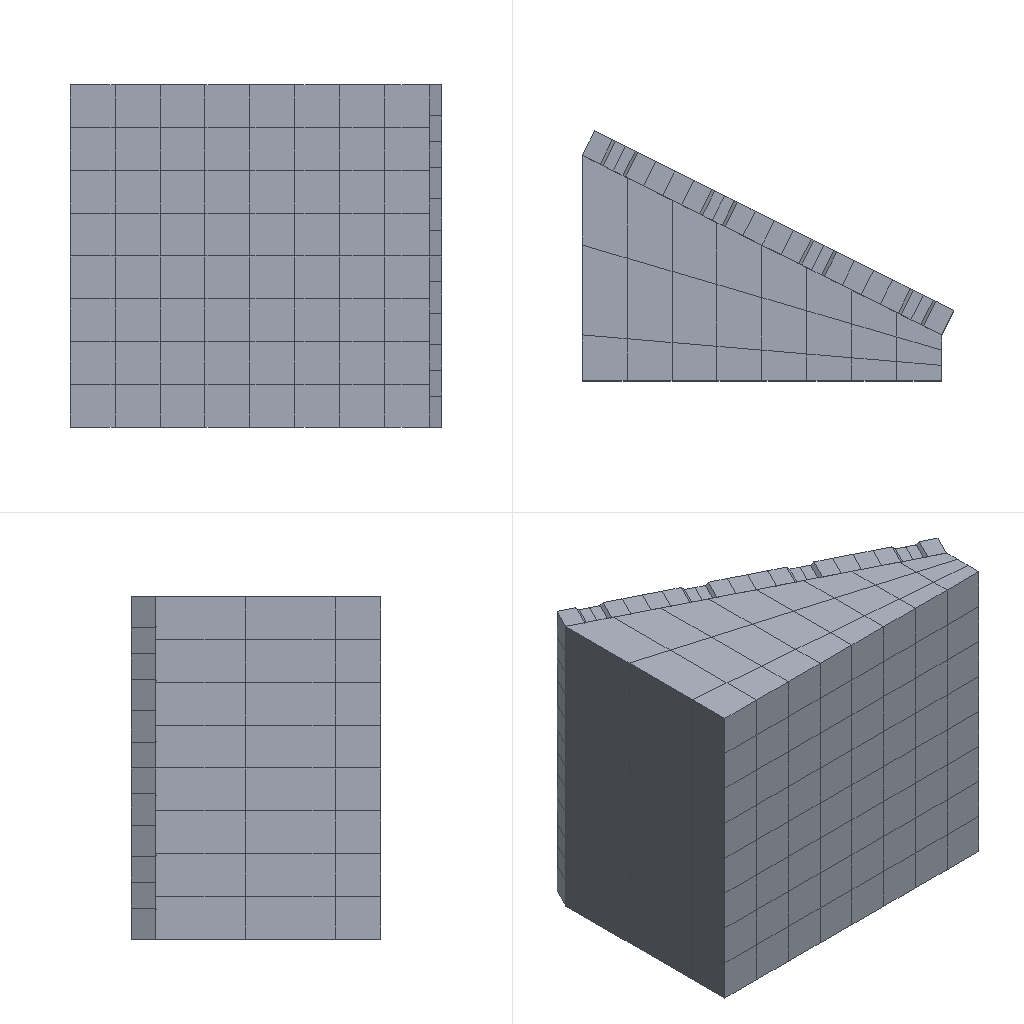Simulation study | abaqus
Set-up summary:
category,name,step,type,value,unit,region
solver,abaqus
solver,version,,,Abaqus/Standard 2020
units,not stated in the deck,,not stated
analysis,deck,,transient,transient
load_step,Step-2,Step-2,transient
load_step,requested,,,1
mesh,nodes,,,3205
mesh,elements,,,1224
element_type,C3D8R,,solid,1224
load,load commands in deck,,count,7
bc,support commands in deck,,count,7
material,HUNNINGTU,,in results
material,S,,in results
check,setup vs results,,match,"per instance, exact: element labels, types and connectivity; labels of the nodes the elements use; coordinates of those nodes at SINGLE_PRECISION in 15 of 31 instance(s)"
Abaqus input file, long lists of numbers shortened, first 402 of 1311 lines:
*Heading
** Job name: Job-2 Model name: Job-9-Copy
** Generated by: Abaqus/CAE 2020
*Preprint, echo=NO, model=NO, history=NO, contact=NO
**
** PARTS
**
*Part, name=BIKONGQIKUAI1
*Node
      1,  -23.409,         -15.,          12.
      2,  -23.409,  -10.17,          12.
** (128 more lines like these left out)
*Element, type=C3D8R
 1,  26,  33,  60,  27,  91,  98, 125,  92
 2,   1,   2,  44,  35,  66,  67, 109, 100
** (46 more lines like these left out)
*Nset, nset=SET-1, generate
   1,  130,    1
*Elset, elset=SET-1, generate
  1,  48,   1
** Section: Section-2-SET-1
*Solid Section, elset=SET-1, material=HUNNINGTU
,
*End Part
**
*Part, name=BIKONGQIKUAI1-COPY
*Node
      1,  0.1705,  -24.319,           0.
      2,  0.1705,  -5.681,           0.
** (62 more lines like these left out)
*Element, type=C3D8R
 1, 21,  3, 29, 25, 53, 35, 61, 57
 2, 22, 32, 30, 20, 54, 64, 62, 52
** (20 more lines like these left out)
*Nset, nset=SET-1, generate
  1,  64,   1
*Elset, elset=SET-1, generate
  1,  22,   1
** Section: Section-3-SET-1
*Solid Section, elset=SET-1, material=HUNNINGTU
,
*End Part
**
*Part, name=BIKONGQIKUAI1-COPY2
*Node
      1,   13.807,  -3.411,          12.
      2,   13.807,  -5.681,          12.
** (24 more lines like these left out)
*Element, type=C3D8R
1,  5, 18,  2,  1,  8, 24, 12, 13
2, 20,  3, 18,  5, 21, 23, 24,  8
** (4 more lines like these left out)
*Nset, nset=TIANCHONG, generate
  1,  26,   1
*Elset, elset=TIANCHONG, generate
 1,  6,  1
** Section: Section-4-TIANCHONG
*Solid Section, elset=TIANCHONG, material=HUNNINGTU
,
*End Part
**
*Part, name=PART-6
*Node
      1,  -157.419,   78.696,         150.
      2,  -137.741,   68.859,         150.
** (323 more lines like these left out)
*Element, type=C3D8R
  1,  82,  83,  92,  91,   1,   2,  11,  10
  2,  83,  84,  93,  92,   2,   3,  12,  11
** (190 more lines like these left out)
*Nset, nset=PART-6-REFPT_, internal
 325,
*Nset, nset=SET-2, generate
   1,  324,    1
*Elset, elset=SET-2, generate
   1,  192,    1
** Section: Section-1-SET-2
*Solid Section, elset=SET-2, material=S
,
*End Part
**
**
** ASSEMBLY
**
*Assembly, name=Assembly
**
*Instance, name=PART-6-1, part=PART-6
*End Instance
**
*Instance, name=BIKONGQIKUAI1-1, part=BIKONGQIKUAI1
-26.827, 13.414, 125.171
-26.827, 13.414, 125.171, -27.292, 14.167, 125.636, 106.047
*End Instance
**
*Instance, name=BIKONGQIKUAI1-COPY-1, part=BIKONGQIKUAI1-COPY
-48.579, 24.288, 150.171
-48.579, 24.288, 150.171, -49.045, 25.041, 150.636, 106.047
*End Instance
**
*Instance, name=BIKONGQIKUAI1-COPY2-1, part=BIKONGQIKUAI1-COPY2
-5.359, -10.734, 124.83
-5.359, -10.734, 124.83, -4.711, -10.333, 125.477, 223.65
*End Instance
**
*Instance, name=BIKONGQIKUAI1-1-LIN-1-2, part=BIKONGQIKUAI1
-26.827, 13.414, 75.171
-26.827, 13.414, 75.171, -27.292, 14.167, 75.636, 106.047
*End Instance
**
*Instance, name=BIKONGQIKUAI1-1-LIN-1-3, part=BIKONGQIKUAI1
-26.827, 13.414, 25.171
-26.827, 13.414, 25.171, -27.292, 14.167, 25.636, 106.047
*End Instance
**
*Instance, name=BIKONGQIKUAI1-1-LIN-2-1, part=BIKONGQIKUAI1
-48.579, 24.288, 100.17
-48.579, 24.288, 100.17, -49.045, 25.041, 100.635, 106.047
*End Instance
**
*Instance, name=BIKONGQIKUAI1-1-LIN-2-2, part=BIKONGQIKUAI1
-48.579, 24.288, 50.171
-48.579, 24.288, 50.171, -49.045, 25.041, 50.636, 106.047
*End Instance
**
*Instance, name=BIKONGQIKUAI1-1-LIN-2-3, part=BIKONGQIKUAI1
-70.331, 35.161, 25.17
-70.331, 35.161, 25.17, -70.797, 35.914, 25.635, 106.047
*End Instance
**
*Instance, name=BIKONGQIKUAI1-1-LIN-3-1, part=BIKONGQIKUAI1
-113.835, 56.909, 125.172
-113.835, 56.909, 125.172, -114.301, 57.662, 125.637, 106.047
*End Instance
**
*Instance, name=BIKONGQIKUAI1-1-LIN-3-2, part=BIKONGQIKUAI1
-92.083, 46.035, 100.171
-92.083, 46.035, 100.171, -92.549, 46.788, 100.636, 106.047
*End Instance
**
*Instance, name=BIKONGQIKUAI1-1-LIN-3-3, part=BIKONGQIKUAI1
-92.083, 46.035, 50.171
-92.083, 46.035, 50.171, -92.549, 46.788, 50.636, 106.047
*End Instance
**
*Instance, name=BIKONGQIKUAI1-1-LIN-4-1, part=BIKONGQIKUAI1
-113.835, 56.909, 75.17
-113.835, 56.909, 75.17, -114.301, 57.662, 75.635, 106.047
*End Instance
**
*Instance, name=BIKONGQIKUAI1-1-LIN-4-2, part=BIKONGQIKUAI1
-135.587, 67.782, 100.171
-135.587, 67.782, 100.171, -136.053, 68.535, 100.636, 106.047
*End Instance
**
*Instance, name=BIKONGQIKUAI1-1-LIN-4-3, part=BIKONGQIKUAI1
-157.34, 78.656, 125.172
-157.34, 78.656, 125.172, -157.805, 79.409, 125.637, 106.047
*End Instance
**
*Instance, name=BIKONGQIKUAI1-1-LIN-2-3-LIN-2-1, part=BIKONGQIKUAI1
-70.331, 35.161, 75.17
-70.331, 35.161, 75.17, -70.797, 35.914, 75.635, 106.047
*End Instance
**
*Instance, name=BIKONGQIKUAI1-1-LIN-2-3-LIN-3-1, part=BIKONGQIKUAI1
-70.331, 35.161, 125.17
-70.331, 35.161, 125.17, -70.797, 35.914, 125.635, 106.047
*End Instance
**
*Instance, name=BIKONGQIKUAI1-1-LIN-4-3-LIN-2-1, part=BIKONGQIKUAI1
-157.34, 78.656, 75.172
-157.34, 78.656, 75.172, -157.805, 79.409, 75.637, 106.047
*End Instance
**
*Instance, name=BIKONGQIKUAI1-1-LIN-4-3-LIN-3-1, part=BIKONGQIKUAI1
-157.34, 78.656, 25.172
-157.34, 78.656, 25.172, -157.805, 79.409, 25.637, 106.047
*End Instance
**
*Instance, name=BIKONGQIKUAI1-1-LIN-4-2-LIN-2-1, part=BIKONGQIKUAI1
-135.587, 67.782, 50.171
-135.587, 67.782, 50.171, -136.053, 68.535, 50.636, 106.047
*End Instance
**
*Instance, name=BIKONGQIKUAI1-1-LIN-4-2-LIN-3-1, part=BIKONGQIKUAI1
-113.835, 56.909, 25.17
-113.835, 56.909, 25.17, -114.301, 57.662, 25.635, 106.047
*End Instance
**
*Instance, name=BIKONGQIKUAI1-COPY-1-LIN-2-1, part=BIKONGQIKUAI1-COPY
-92.083, 46.035, 150.173
-92.083, 46.035, 150.173, -92.549, 46.788, 150.638, 106.047
*End Instance
**
*Instance, name=BIKONGQIKUAI1-COPY-1-LIN-3-1, part=BIKONGQIKUAI1-COPY
-135.587, 67.782, 150.173
-135.587, 67.782, 150.173, -136.053, 68.535, 150.638, 106.047
*End Instance
**
*Instance, name=BIKONGQIKUAI1-COPY-1-LIN-4-1, part=BIKONGQIKUAI1-COPY
-130.222, 78.516, -0.1725
-130.222, 78.516, -0.1725, -129.757, 77.763, 0.2929, 106.047
*End Instance
**
*Instance, name=BIKONGQIKUAI1-COPY-1-LIN-4-1-LIN-2-1, part=BIKONGQIKUAI1-COPY
-86.718, 56.769, -0.1725
-86.718, 56.769, -0.1725, -86.252, 56.016, 0.2929, 106.047
*End Instance
**
*Instance, name=BIKONGQIKUAI1-COPY-1-LIN-4-1-LIN-3-1, part=BIKONGQIKUAI1-COPY
-43.214, 35.021, -0.1715
-43.214, 35.021, -0.1715, -42.748, 34.268, 0.2939, 106.047
*End Instance
**
*Instance, name=BIKONGQIKUAI1-COPY2-1-LIN-2-1, part=BIKONGQIKUAI1-COPY2
-5.359, -10.734, 74.829
-5.359, -10.734, 74.829, -4.711, -10.333, 75.477, 223.65
*End Instance
**
*Instance, name=BIKONGQIKUAI1-COPY2-1-LIN-3-1, part=BIKONGQIKUAI1-COPY2
-5.359, -10.734, 24.829
-5.359, -10.734, 24.829, -4.711, -10.333, 25.477, 223.65
*End Instance
**
*Instance, name=BIKONGQIKUAI1-COPY2-1-LIN-3-1-LIN-2-1, part=BIKONGQIKUAI1-COPY2
-146.608, 100.123, 124.83
-146.608, 100.123, 124.83, -146.143, 99.37, 125.296, 106.047
*End Instance
**
*Instance, name=BIKONGQIKUAI1-COPY2-1-LIN-3--LIN-2-1, part=BIKONGQIKUAI1-COPY2
-146.608, 100.123, 74.831
-146.608, 100.123, 74.831, -146.143, 99.37, 75.296, 106.047
*End Instance
**
*Instance, name=BIKONGQIKUAI1-COPY2-1-LIN-3--LIN-3-1, part=BIKONGQIKUAI1-COPY2
-146.608, 100.123, 24.831
-146.608, 100.123, 24.831, -146.143, 99.37, 25.296, 106.047
*End Instance
**
*Nset, nset=DIMIAN, instance=PART-6-1, generate
 244,  324,    1
*Elset, elset=DIMIAN, instance=PART-6-1, generate
 129,  192,    1
*Nset, nset=SET-5, instance=BIKONGQIKUAI1-1
  4,  5, 30, 31, 69, 70, 95, 96
*Nset, nset=SET-5, instance=BIKONGQIKUAI1-1-LIN-1-3
 14, 15, 19, 20, 79, 80, 84, 85
*Nset, nset=SET-5, instance=BIKONGQIKUAI1-COPY-1-LIN-4-1-LIN-2-1
  1,  2, 18, 33, 34, 50
*Nset, nset=SET-5, instance=BIKONGQIKUAI1-1-LIN-2-3
 14, 15, 19, 20, 79, 80, 84, 85
*Nset, nset=SET-5, instance=BIKONGQIKUAI1-1-LIN-2-3-LIN-3-1
  4,  5, 30, 31, 69, 70, 95, 96
*Nset, nset=SET-5, instance=BIKONGQIKUAI1-1-LIN-4-2-LIN-3-1
 14, 15, 19, 20, 79, 80, 84, 85
*Nset, nset=SET-5, instance=BIKONGQIKUAI1-1-LIN-4-3
  4,  5, 30, 31, 69, 70, 95, 96
*Nset, nset=SET-5, instance=BIKONGQIKUAI1-1-LIN-4-3-LIN-3-1
 14, 15, 19, 20, 79, 80, 84, 85
*Nset, nset=SET-5, instance=BIKONGQIKUAI1-COPY-1
  1,  2, 18, 33, 34, 50
*Nset, nset=SET-5, instance=BIKONGQIKUAI1-COPY-1-LIN-3-1
  1,  2, 18, 33, 34, 50
*Nset, nset=SET-5, instance=BIKONGQIKUAI1-1-LIN-3-1
  4,  5, 30, 31, 69, 70, 95, 96
*Nset, nset=SET-5, instance=BIKONGQIKUAI1-COPY-1-LIN-2-1
  1,  2, 18, 33, 34, 50
*Nset, nset=SET-5, instance=BIKONGQIKUAI1-COPY-1-LIN-4-1-LIN-3-1
  1,  2, 18, 33, 34, 50
*Nset, nset=SET-5, instance=BIKONGQIKUAI1-COPY-1-LIN-4-1
  1,  2, 18, 33, 34, 50
*Elset, elset=SET-5, instance=BIKONGQIKUAI1-1
  4, 23
*Elset, elset=SET-5, instance=BIKONGQIKUAI1-1-LIN-1-3
 13, 20
*Elset, elset=SET-5, instance=BIKONGQIKUAI1-COPY-1-LIN-4-1-LIN-2-1
 17, 20
*Elset, elset=SET-5, instance=BIKONGQIKUAI1-1-LIN-2-3
 13, 20
*Elset, elset=SET-5, instance=BIKONGQIKUAI1-1-LIN-2-3-LIN-3-1
  4, 23
*Elset, elset=SET-5, instance=BIKONGQIKUAI1-1-LIN-4-2-LIN-3-1
 13, 20
*Elset, elset=SET-5, instance=BIKONGQIKUAI1-1-LIN-4-3
  4, 23
*Elset, elset=SET-5, instance=BIKONGQIKUAI1-1-LIN-4-3-LIN-3-1
 13, 20
*Elset, elset=SET-5, instance=BIKONGQIKUAI1-COPY-1
 17, 20
*Elset, elset=SET-5, instance=BIKONGQIKUAI1-COPY-1-LIN-3-1
 17, 20
*Elset, elset=SET-5, instance=BIKONGQIKUAI1-1-LIN-3-1
  4, 23
*Elset, elset=SET-5, instance=BIKONGQIKUAI1-COPY-1-LIN-2-1
 17, 20
*Elset, elset=SET-5, instance=BIKONGQIKUAI1-COPY-1-LIN-4-1-LIN-3-1
 17, 20
*Elset, elset=SET-5, instance=BIKONGQIKUAI1-COPY-1-LIN-4-1
 17, 20
*Nset, nset=SET-6, instance=BIKONGQIKUAI1-1
  6, 13, 71, 78
*Nset, nset=SET-6, instance=BIKONGQIKUAI1-1-LIN-1-2
  5,  6, 13, 14, 70, 71, 78, 79
*Nset, nset=SET-6, instance=BIKONGQIKUAI1-1-LIN-1-3
  6, 13, 71, 78
*Nset, nset=Set-97, instance=BIKONGQIKUAI1-1-LIN-1-3
 14, 15, 19, 20, 79, 80, 84, 85
*Nset, nset=Set-97, instance=BIKONGQIKUAI1-COPY-1-LIN-4-1-LIN-3-1
  1,  2, 18, 33, 34, 50
*Nset, nset=Set-97, instance=BIKONGQIKUAI1-1-LIN-2-3
 14, 15, 19, 20, 79, 80, 84, 85
*Nset, nset=Set-97, instance=BIKONGQIKUAI1-COPY-1-LIN-4-1-LIN-2-1
  1,  2, 18, 33, 34, 50
*Nset, nset=Set-97, instance=BIKONGQIKUAI1-1-LIN-2-3-LIN-3-1
  4,  5, 30, 31, 69, 70, 95, 96
*Nset, nset=Set-97, instance=BIKONGQIKUAI1-1-LIN-4-2-LIN-3-1
 14, 15, 19, 20, 79, 80, 84, 85
*Nset, nset=Set-97, instance=BIKONGQIKUAI1-1-LIN-4-3-LIN-3-1
 14, 15, 19, 20, 79, 80, 84, 85
*Nset, nset=Set-97, instance=BIKONGQIKUAI1-COPY-1
  1,  2, 18, 33, 34, 50
*Nset, nset=Set-97, instance=BIKONGQIKUAI1-1-LIN-4-3
  4,  5, 30, 31, 69, 70, 95, 96
*Nset, nset=Set-97, instance=BIKONGQIKUAI1-COPY-1-LIN-3-1
  1,  2, 18, 33, 34, 50
*Nset, nset=Set-97, instance=BIKONGQIKUAI1-COPY-1-LIN-4-1
  1,  2, 18, 33, 34, 50
*Nset, nset=Set-97, instance=BIKONGQIKUAI1-1-LIN-3-1
  4,  5, 30, 31, 69, 70, 95, 96
*Nset, nset=Set-97, instance=BIKONGQIKUAI1-1
  4,  5, 30, 31, 69, 70, 95, 96
*Nset, nset=Set-97, instance=BIKONGQIKUAI1-COPY-1-LIN-2-1
  1,  2, 18, 33, 34, 50
*Nset, nset=Set-98, instance=BIKONGQIKUAI1-1-LIN-1-3
  5,  6, 13, 14, 70, 71, 78, 79
*Nset, nset=Set-98, instance=BIKONGQIKUAI1-COPY2-1-LIN-3-1
 14, 15, 16, 17, 25, 26
*Nset, nset=Set-98, instance=BIKONGQIKUAI1-1-LIN-1-2
  5,  6, 13, 14, 70, 71, 78, 79
*Nset, nset=Set-98, instance=BIKONGQIKUAI1-COPY2-1-LIN-2-1
 14, 15, 16, 17, 25, 26
*Nset, nset=Set-98, instance=BIKONGQIKUAI1-1
  5,  6, 13, 14, 70, 71, 78, 79
*Nset, nset=Set-98, instance=BIKONGQIKUAI1-COPY2-1
 14, 15, 16, 17, 25, 26
*Nset, nset=Set-99, instance=BIKONGQIKUAI1-1-LIN-1-3
  5,  6, 13, 14, 70, 71, 78, 79
*Nset, nset=Set-99, instance=BIKONGQIKUAI1-COPY2-1-LIN-3-1
 14, 15, 16, 17, 25, 26
*Nset, nset=Set-99, instance=BIKONGQIKUAI1-1-LIN-1-2
  5,  6, 13, 14, 70, 71, 78, 79
*Nset, nset=Set-99, instance=BIKONGQIKUAI1-COPY2-1-LIN-3-1-LIN-2-1
 14, 15, 16, 17, 25, 26
*Nset, nset=Set-99, instance=BIKONGQIKUAI1-COPY2-1-LIN-2-1
 14, 15, 16, 17, 25, 26
*Nset, nset=Set-99, instance=BIKONGQIKUAI1-1-LIN-4-3-LIN-3-1
 20, 21, 29, 30, 85, 86, 94, 95
*Nset, nset=Set-99, instance=BIKONGQIKUAI1-1-LIN-4-3
 29, 30, 94, 95
*Nset, nset=Set-99, instance=BIKONGQIKUAI1-COPY2-1-LIN-3--LIN-3-1
 14, 15, 16, 17, 25, 26
*Nset, nset=Set-99, instance=BIKONGQIKUAI1-1
  5,  6, 13, 14, 70, 71, 78, 79
*Nset, nset=Set-99, instance=BIKONGQIKUAI1-COPY2-1-LIN-3--LIN-2-1
 14, 15, 16, 17, 25, 26
*Nset, nset=Set-99, instance=BIKONGQIKUAI1-1-LIN-4-3-LIN-2-1
 29, 30, 94, 95
*Nset, nset=Set-99, instance=BIKONGQIKUAI1-COPY2-1
 14, 15, 16, 17, 25, 26
*Elset, elset=_POMIAN_S2, internal, instance=PART-6-1, generate
  1,  64,   1
*Elset, elset=_SURF-3_S2, internal, instance=BIKONGQIKUAI1-1-LIN-3-2, generate
  1,  48,   1
*Elset, elset=_SURF-3_S2, internal, instance=BIKONGQIKUAI1-1-LIN-3-3, generate
  1,  48,   1
*Elset, elset=_SURF-3_S2, internal, instance=BIKONGQIKUAI1-1-LIN-4-1, generate
  1,  48,   1
*Elset, elset=_SURF-4_S2, internal, instance=BIKONGQIKUAI1-1-LIN-2-3-LIN-2-1, generate
  1,  48,   1
*Elset, elset=_SURF-5_S2, internal, instance=BIKONGQIKUAI1-1-LIN-3-2, generate
  1,  48,   1
*Elset, elset=_SURF-5_S2, internal, instance=BIKONGQIKUAI1-1-LIN-3-3, generate
  1,  48,   1
*Elset, elset=_SURF-5_S2, internal, instance=BIKONGQIKUAI1-1-LIN-4-1, generate
  1,  48,   1
*Elset, elset=_SURF-5_S2, internal, instance=BIKONGQIKUAI1-1-LIN-2-3-LIN-2-1, generate
  1,  48,   1
*Nset, nset="_T-Datum csys-2", internal, instance=BIKONGQIKUAI1-1
  6, 13, 71, 78
*Nset, nset="_T-Datum csys-2", internal, instance=BIKONGQIKUAI1-1-LIN-1-2
  5,  6, 13, 14, 70, 71, 78, 79
*Nset, nset="_T-Datum csys-2", internal, instance=BIKONGQIKUAI1-1-LIN-1-3
  6, 13, 71, 78
*Elset, elset=_ZHUANDIMIAN_S1, internal, instance=BIKONGQIKUAI1-COPY-1-LIN-2-1, generate
  1,  22,   1
*Elset, elset=_ZHUANDIMIAN_S1, internal, instance=BIKONGQIKUAI1-COPY2-1-LIN-2-1, generate
 1,  4,  1
*Elset, elset=_ZHUANDIMIAN_S1, internal, instance=BIKONGQIKUAI1-COPY-1-LIN-3-1, generate
  1,  22,   1
*Elset, elset=_ZHUANDIMIAN_S1, internal, instance=BIKONGQIKUAI1-COPY-1, generate
  1,  22,   1
*Elset, elset=_ZHUANDIMIAN_S1, internal, instance=BIKONGQIKUAI1-COPY2-1-LIN-3-1, generate
Last 654 lines:
*Elset, elset=_Surf-90_S1, internal, instance=BIKONGQIKUAI1-COPY2-1-LIN-3-1-LIN-2-1, generate
 1,  4,  1
*Elset, elset=_Surf-90_S1, internal, instance=BIKONGQIKUAI1-1-LIN-2-1, generate
  1,  48,   1
*Elset, elset=_Surf-90_S1, internal, instance=BIKONGQIKUAI1-1-LIN-3-2, generate
  1,  48,   1
*Elset, elset=_Surf-90_S1, internal, instance=BIKONGQIKUAI1-1-LIN-4-3-LIN-3-1, generate
  1,  48,   1
*Elset, elset=_Surf-90_S1, internal, instance=BIKONGQIKUAI1-1-LIN-4-3, generate
  1,  48,   1
*Elset, elset=_Surf-90_S1, internal, instance=BIKONGQIKUAI1-COPY2-1-LIN-3--LIN-3-1, generate
 1,  4,  1
*Elset, elset=_Surf-90_S1, internal, instance=BIKONGQIKUAI1-COPY-1-LIN-4-1-LIN-3-1, generate
  1,  22,   1
*Elset, elset=_Surf-90_S1, internal, instance=BIKONGQIKUAI1-1, generate
  1,  48,   1
*Elset, elset=_Surf-90_S1, internal, instance=BIKONGQIKUAI1-1-LIN-3-1, generate
  1,  48,   1
*Elset, elset=_Surf-90_S1, internal, instance=BIKONGQIKUAI1-1-LIN-4-3-LIN-2-1, generate
  1,  48,   1
*Elset, elset=_Surf-90_S1, internal, instance=BIKONGQIKUAI1-1-LIN-4-2, generate
  1,  48,   1
*Elset, elset=_Surf-90_S1, internal, instance=BIKONGQIKUAI1-COPY2-1-LIN-3--LIN-2-1, generate
 1,  4,  1
*Elset, elset=_Surf-90_S1, internal, instance=BIKONGQIKUAI1-1-LIN-3-3, generate
  1,  48,   1
*Elset, elset=_Surf-90_S1, internal, instance=BIKONGQIKUAI1-1-LIN-4-2-LIN-2-1, generate
  1,  48,   1
*Elset, elset=_Surf-90_S1, internal, instance=BIKONGQIKUAI1-1-LIN-2-3-LIN-2-1, generate
  1,  48,   1
*Elset, elset=_Surf-90_S1, internal, instance=BIKONGQIKUAI1-COPY-1-LIN-4-1, generate
  1,  22,   1
*Elset, elset=_Surf-90_S5, internal, instance=BIKONGQIKUAI1-COPY2-1-LIN-3-1-LIN-2-1
 5, 6
*Elset, elset=_Surf-90_S5, internal, instance=BIKONGQIKUAI1-COPY2-1-LIN-3--LIN-3-1
 5, 6
*Elset, elset=_Surf-90_S5, internal, instance=BIKONGQIKUAI1-COPY2-1-LIN-3--LIN-2-1
 5, 6
*Elset, elset=_Surf-90_S2, internal, instance=BIKONGQIKUAI1-COPY-1, generate
  1,  22,   1
*Elset, elset=_Surf-90_S2, internal, instance=BIKONGQIKUAI1-COPY2-1-LIN-2-1, generate
 1,  4,  1
*Elset, elset=_Surf-90_S2, internal, instance=BIKONGQIKUAI1-COPY-1-LIN-3-1, generate
  1,  22,   1
*Elset, elset=_Surf-90_S2, internal, instance=BIKONGQIKUAI1-COPY-1-LIN-2-1, generate
  1,  22,   1
*Elset, elset=_Surf-90_S2, internal, instance=BIKONGQIKUAI1-COPY2-1, generate
 1,  4,  1
*Elset, elset=_Surf-90_S2, internal, instance=BIKONGQIKUAI1-COPY2-1-LIN-3-1, generate
 1,  4,  1
*Elset, elset=_Surf-90_S3, internal, instance=BIKONGQIKUAI1-COPY2-1-LIN-2-1
 5, 6
*Elset, elset=_Surf-90_S3, internal, instance=BIKONGQIKUAI1-COPY2-1
 5, 6
*Elset, elset=_Surf-90_S3, internal, instance=BIKONGQIKUAI1-COPY2-1-LIN-3-1
 5, 6
*Surface, type=ELEMENT, name=Surf-90
_Surf-90_S1, S1
_Surf-90_S5, S5
_Surf-90_S2, S2
_Surf-90_S3, S3
*Elset, elset=_Surf-91_S1, internal, instance=BIKONGQIKUAI1-1-LIN-2-2
  1,  2,  3,  4,  5,  6,  7,  8,  9, 10, 11, 12, 15, 16, 18, 19
 20, 21, 22, 24, 25, 26, 27, 28, 29, 30, 31, 32, 33, 34, 35, 36
** (1 more lines like these left out)
*Elset, elset=_Surf-91_S1, internal, instance=BIKONGQIKUAI1-1-LIN-1-3, generate
  1,  48,   1
*Elset, elset=_Surf-91_S1, internal, instance=BIKONGQIKUAI1-1-LIN-2-1
  1,  2,  3,  4,  5,  6,  7,  8,  9, 10, 11, 12, 15, 16, 18, 19
 20, 21, 22, 24, 25, 26, 27, 28, 29, 30, 31, 32, 33, 34, 35, 36
** (1 more lines like these left out)
*Elset, elset=_Surf-91_S1, internal, instance=BIKONGQIKUAI1-1-LIN-1-2, generate
  1,  48,   1
*Elset, elset=_Surf-91_S1, internal, instance=BIKONGQIKUAI1-COPY-1-LIN-4-1-LIN-3-1
  1,  2,  3,  4,  6,  7,  8,  9, 10, 11, 12, 13, 14, 15, 16, 17
 18, 19, 20, 22
*Elset, elset=_Surf-91_S1, internal, instance=BIKONGQIKUAI1-1, generate
  1,  48,   1
*Elset, elset=_Surf-91_S2, internal, instance=BIKONGQIKUAI1-COPY-1
  1,  2,  3,  4,  6,  7,  8,  9, 10, 11, 12, 13, 14, 15, 16, 17
 18, 19, 20, 22
*Elset, elset=_Surf-91_S2, internal, instance=BIKONGQIKUAI1-COPY2-1-LIN-2-1, generate
 1,  4,  1
*Elset, elset=_Surf-91_S2, internal, instance=BIKONGQIKUAI1-COPY2-1-LIN-3-1, generate
 1,  4,  1
*Elset, elset=_Surf-91_S2, internal, instance=BIKONGQIKUAI1-COPY2-1, generate
 1,  4,  1
*Elset, elset=_Surf-91_S3, internal, instance=BIKONGQIKUAI1-COPY2-1-LIN-2-1
 5, 6
*Elset, elset=_Surf-91_S3, internal, instance=BIKONGQIKUAI1-COPY2-1-LIN-3-1
 5, 6
*Elset, elset=_Surf-91_S3, internal, instance=BIKONGQIKUAI1-COPY2-1
 5, 6
*Surface, type=ELEMENT, name=Surf-91
_Surf-91_S1, S1
_Surf-91_S2, S2
_Surf-91_S3, S3
*Elset, elset=_Surf-92_S1, internal, instance=BIKONGQIKUAI1-1-LIN-2-2
  1, 13, 14, 15, 17, 22, 23, 24, 25, 27, 29, 34, 35, 36, 41
*Elset, elset=_Surf-92_S1, internal, instance=BIKONGQIKUAI1-COPY-1-LIN-4-1-LIN-3-1
  1,  5, 10, 11, 16, 21
*Elset, elset=_Surf-92_S1, internal, instance=BIKONGQIKUAI1-1-LIN-2-3, generate
  1,  48,   1
*Elset, elset=_Surf-92_S1, internal, instance=BIKONGQIKUAI1-1-LIN-2-3-LIN-3-1, generate
  1,  48,   1
*Elset, elset=_Surf-92_S1, internal, instance=BIKONGQIKUAI1-COPY-1-LIN-4-1-LIN-2-1
  2,  3,  4,  6,  7,  8,  9, 12, 13, 14, 15, 17, 19, 22
*Elset, elset=_Surf-92_S1, internal, instance=BIKONGQIKUAI1-1-LIN-2-1
  1, 13, 14, 15, 17, 22, 23, 24, 25, 27, 29, 34, 35, 36, 41
*Elset, elset=_Surf-92_S1, internal, instance=BIKONGQIKUAI1-1-LIN-3-2
  2,  3,  4,  5,  6,  7,  8,  9, 10, 11, 12, 16, 18, 19, 20, 21
 26, 28, 30, 31, 32, 33, 35, 37, 38, 39, 40, 43, 44, 45, 46, 47
*Elset, elset=_Surf-92_S1, internal, instance=BIKONGQIKUAI1-1-LIN-3-3
  2,  3,  4,  5,  6,  7,  8,  9, 10, 11, 12, 16, 18, 19, 20, 21
 26, 28, 30, 31, 32, 33, 35, 37, 38, 39, 40, 43, 44, 45, 46, 47
*Elset, elset=_Surf-92_S1, internal, instance=BIKONGQIKUAI1-1-LIN-2-3-LIN-2-1, generate
  1,  48,   1
*Elset, elset=_Surf-92_S2, internal, instance=BIKONGQIKUAI1-COPY-1
  1,  5, 10, 11, 16, 21
*Elset, elset=_Surf-92_S2, internal, instance=BIKONGQIKUAI1-COPY-1-LIN-2-1
  2,  3,  4,  6,  7,  8,  9, 12, 13, 14, 15, 17, 19, 22
*Surface, type=ELEMENT, name=Surf-92
_Surf-92_S1, S1
_Surf-92_S2, S2
*Elset, elset=_Surf-93_S1, internal, instance=BIKONGQIKUAI1-1-LIN-3-3
  1,  2, 11, 12, 13, 14, 15, 17, 22, 23, 24, 25, 27, 29, 30, 34
 35, 36, 41, 48
*Elset, elset=_Surf-93_S1, internal, instance=BIKONGQIKUAI1-COPY-1-LIN-4-1-LIN-2-1
  1,  5,  6,  7, 10, 11, 16, 18, 20, 21
*Elset, elset=_Surf-93_S1, internal, instance=BIKONGQIKUAI1-1-LIN-4-2-LIN-3-1, generate
  1,  48,   1
*Elset, elset=_Surf-93_S1, internal, instance=BIKONGQIKUAI1-1-LIN-4-1, generate
  1,  48,   1
*Elset, elset=_Surf-93_S1, internal, instance=BIKONGQIKUAI1-1-LIN-3-2
  1,  2, 11, 12, 13, 14, 15, 17, 22, 23, 24, 25, 27, 29, 30, 34
 35, 36, 41, 48
*Elset, elset=_Surf-93_S1, internal, instance=BIKONGQIKUAI1-1-LIN-3-1, generate
  1,  48,   1
*Elset, elset=_Surf-93_S1, internal, instance=BIKONGQIKUAI1-1-LIN-4-2
  3,  4,  5,  6,  7,  8,  9, 10, 16, 18, 19, 20, 21, 26, 31, 32
 33, 37, 40, 43, 44, 45, 46
*Elset, elset=_Surf-93_S1, internal, instance=BIKONGQIKUAI1-1-LIN-4-2-LIN-2-1
  3,  4,  5,  6,  7,  8,  9, 10, 16, 18, 19, 20, 21, 26, 31, 32
 33, 37, 40, 43, 44, 45, 46
*Elset, elset=_Surf-93_S1, internal, instance=BIKONGQIKUAI1-COPY-1-LIN-4-1
  2,  3,  4,  8,  9, 12, 13, 14, 15, 17, 19, 22
*Elset, elset=_Surf-93_S2, internal, instance=BIKONGQIKUAI1-COPY-1-LIN-3-1
  2,  3,  4,  8,  9, 12, 13, 14, 15, 17, 19, 22
*Elset, elset=_Surf-93_S2, internal, instance=BIKONGQIKUAI1-COPY-1-LIN-2-1
  1,  5,  6,  7, 10, 11, 16, 18, 20, 21
*Surface, type=ELEMENT, name=Surf-93
_Surf-93_S1, S1
_Surf-93_S2, S2
*Elset, elset=_Surf-94_S1, internal, instance=BIKONGQIKUAI1-1-LIN-4-2
  1,  2, 11, 12, 13, 14, 15, 17, 22, 23, 24, 25, 27, 28, 29, 30
 34, 35, 36, 38, 41, 42, 46, 47, 48
*Elset, elset=_Surf-94_S1, internal, instance=BIKONGQIKUAI1-1-LIN-4-3, generate
  1,  48,   1
*Elset, elset=_Surf-94_S1, internal, instance=BIKONGQIKUAI1-1-LIN-4-3-LIN-3-1, generate
  1,  48,   1
*Elset, elset=_Surf-94_S1, internal, instance=BIKONGQIKUAI1-COPY2-1-LIN-3-1-LIN-2-1, generate
 1,  4,  1
*Elset, elset=_Surf-94_S1, internal, instance=BIKONGQIKUAI1-COPY2-1-LIN-3--LIN-3-1, generate
 1,  4,  1
*Elset, elset=_Surf-94_S1, internal, instance=BIKONGQIKUAI1-1-LIN-4-3-LIN-2-1, generate
  1,  48,   1
*Elset, elset=_Surf-94_S1, internal, instance=BIKONGQIKUAI1-COPY2-1-LIN-3--LIN-2-1, generate
 1,  4,  1
*Elset, elset=_Surf-94_S1, internal, instance=BIKONGQIKUAI1-1-LIN-4-2-LIN-2-1
  1,  2, 11, 12, 13, 14, 15, 17, 22, 23, 24, 25, 27, 28, 29, 30
 34, 35, 36, 38, 41, 42, 46, 47, 48
*Elset, elset=_Surf-94_S1, internal, instance=BIKONGQIKUAI1-COPY-1-LIN-4-1
  1,  5,  6,  7, 10, 11, 16, 18, 20, 21
*Elset, elset=_Surf-94_S5, internal, instance=BIKONGQIKUAI1-COPY2-1-LIN-3-1-LIN-2-1
 5, 6
*Elset, elset=_Surf-94_S5, internal, instance=BIKONGQIKUAI1-COPY2-1-LIN-3--LIN-3-1
 5, 6
*Elset, elset=_Surf-94_S5, internal, instance=BIKONGQIKUAI1-COPY2-1-LIN-3--LIN-2-1
 5, 6
*Elset, elset=_Surf-94_S2, internal, instance=BIKONGQIKUAI1-COPY-1-LIN-3-1
  1,  5,  6,  7, 10, 11, 16, 18, 20, 21
*Surface, type=ELEMENT, name=Surf-94
_Surf-94_S1, S1
_Surf-94_S5, S5
_Surf-94_S2, S2
*Elset, elset=_Surf-95_S1, internal, instance=BIKONGQIKUAI1-1-LIN-3-3
  1,  2, 14, 15, 17, 22, 23, 24, 25, 29, 30, 35, 36, 41, 48
*Elset, elset=_Surf-95_S1, internal, instance=BIKONGQIKUAI1-1-LIN-4-2-LIN-3-1
  1,  2,  3,  4,  5,  6, 15, 16, 17, 19, 23, 24, 28, 29, 30, 31
 32, 35, 37, 43, 45
*Elset, elset=_Surf-95_S1, internal, instance=BIKONGQIKUAI1-1-LIN-3-2
  1,  2, 11, 12, 13, 14, 15, 17, 22, 23, 24, 25, 27, 29, 30, 34
 35, 36, 41, 48
*Elset, elset=_Surf-95_S1, internal, instance=BIKONGQIKUAI1-1-LIN-4-1, generate
  1,  48,   1
*Elset, elset=_Surf-95_S1, internal, instance=BIKONGQIKUAI1-1-LIN-3-1
  7,  8,  9, 10, 11, 12, 13, 14, 18, 20, 21, 22, 26, 27, 33, 34
 36, 38, 40, 41, 46, 47, 48
*Elset, elset=_Surf-95_S1, internal, instance=BIKONGQIKUAI1-1-LIN-4-2
  3,  4,  5,  6,  7,  8,  9, 10, 16, 18, 19, 20, 21, 26, 31, 32
 33, 37, 40, 43, 44, 45, 46
*Elset, elset=_Surf-95_S1, internal, instance=BIKONGQIKUAI1-1-LIN-4-2-LIN-2-1
  3,  4,  5,  6,  8,  9, 10, 16, 18, 19, 26, 31, 32, 33, 37, 40
 43, 44, 45, 46
*Surface, type=ELEMENT, name=Surf-95
_Surf-95_S1, S1
*Elset, elset=_Surf-96_S1, internal, instance=BIKONGQIKUAI1-1-LIN-3-3
 17, 23
*Elset, elset=_Surf-96_S1, internal, instance=BIKONGQIKUAI1-1-LIN-3-2
 13, 14
*Elset, elset=_Surf-96_S1, internal, instance=BIKONGQIKUAI1-1-LIN-4-1
  1,  2,  3,  6,  7,  8,  9, 11, 12, 15, 16, 18, 19, 21, 22, 24
 25, 26, 27, 28, 29, 30, 31, 32, 33, 34, 35, 36, 37, 38, 39, 40
** (1 more lines like these left out)
*Elset, elset=_Surf-96_S1, internal, instance=BIKONGQIKUAI1-1-LIN-4-2
 10, 20
*Elset, elset=_Surf-96_S1, internal, instance=BIKONGQIKUAI1-1-LIN-4-2-LIN-2-1
 4, 5
*Surface, type=ELEMENT, name=Surf-96
_Surf-96_S1, S1
*Elset, elset=_Surf-97_S1, internal, instance=BIKONGQIKUAI1-1-LIN-4-1, generate
  1,  48,   1
*Surface, type=ELEMENT, name=Surf-97
_Surf-97_S1, S1
*Elset, elset=_Surf-98_S1, internal, instance=BIKONGQIKUAI1-1-LIN-3-1, generate
  1,  48,   1
*Surface, type=ELEMENT, name=Surf-98
_Surf-98_S1, S1
*Elset, elset=_Surf-99_S1, internal, instance=BIKONGQIKUAI1-1-LIN-4-2-LIN-3-1, generate
  1,  48,   1
*Surface, type=ELEMENT, name=Surf-99
_Surf-99_S1, S1
*Elset, elset=_Surf-100_S1, internal, instance=BIKONGQIKUAI1-1-LIN-4-2, generate
  1,  48,   1
*Surface, type=ELEMENT, name=Surf-100
_Surf-100_S1, S1
*Elset, elset=_Surf-101_S1, internal, instance=BIKONGQIKUAI1-1-LIN-4-2-LIN-2-1, generate
  1,  48,   1
*Surface, type=ELEMENT, name=Surf-101
_Surf-101_S1, S1
*Elset, elset=_Surf-102_S1, internal, instance=BIKONGQIKUAI1-1-LIN-3-2, generate
  1,  48,   1
*Surface, type=ELEMENT, name=Surf-102
_Surf-102_S1, S1
*Elset, elset=_Surf-103_S1, internal, instance=BIKONGQIKUAI1-1-LIN-3-3, generate
  1,  48,   1
*Surface, type=ELEMENT, name=Surf-103
_Surf-103_S1, S1
*Elset, elset=_Surf-104_S1, internal, instance=BIKONGQIKUAI1-1-LIN-1-3, generate
  1,  48,   1
*Elset, elset=_Surf-104_S1, internal, instance=BIKONGQIKUAI1-1-LIN-1-2, generate
  1,  48,   1
*Elset, elset=_Surf-104_S1, internal, instance=BIKONGQIKUAI1-1, generate
  1,  48,   1
*Surface, type=ELEMENT, name=Surf-104
_Surf-104_S1, S1
*Elset, elset=_Surf-105_S1, internal, instance=BIKONGQIKUAI1-1-LIN-1-3, generate
  1,  48,   1
*Elset, elset=_Surf-105_S1, internal, instance=BIKONGQIKUAI1-1-LIN-1-2, generate
  1,  48,   1
*Elset, elset=_Surf-105_S1, internal, instance=BIKONGQIKUAI1-1-LIN-2-1, generate
  1,  48,   1
*Elset, elset=_Surf-105_S1, internal, instance=BIKONGQIKUAI1-1, generate
  1,  48,   1
*Elset, elset=_Surf-105_S1, internal, instance=BIKONGQIKUAI1-1-LIN-2-2, generate
  1,  48,   1
*Surface, type=ELEMENT, name=Surf-105
_Surf-105_S1, S1
*Elset, elset=_Surf-106_S1, internal, instance=BIKONGQIKUAI1-1, generate
  1,  48,   1
*Elset, elset=_Surf-106_S1, internal, instance=BIKONGQIKUAI1-1-LIN-1-2, generate
  1,  48,   1
*Elset, elset=_Surf-106_S1, internal, instance=BIKONGQIKUAI1-1-LIN-2-1, generate
  1,  48,   1
*Elset, elset=_Surf-106_S1, internal, instance=BIKONGQIKUAI1-1-LIN-2-2, generate
  1,  48,   1
*Elset, elset=_Surf-106_S1, internal, instance=BIKONGQIKUAI1-1-LIN-1-3, generate
  1,  48,   1
*Surface, type=ELEMENT, name=Surf-106
_Surf-106_S1, S1
*Elset, elset=_ZHUANDIMIAN_S2_1, internal, instance=BIKONGQIKUAI1-1, generate
  1,  48,   1
*Elset, elset=_ZHUANDIMIAN_S2_1, internal, instance=BIKONGQIKUAI1-1-LIN-1-2, generate
  1,  48,   1
*Elset, elset=_ZHUANDIMIAN_S2_1, internal, instance=BIKONGQIKUAI1-1-LIN-3-2, generate
  1,  48,   1
*Elset, elset=_ZHUANDIMIAN_S2_1, internal, instance=BIKONGQIKUAI1-1-LIN-2-3, generate
  1,  48,   1
*Elset, elset=_ZHUANDIMIAN_S2_1, internal, instance=BIKONGQIKUAI1-COPY-1-LIN-4-1-LIN-2-1, generate
  1,  22,   1
*Elset, elset=_ZHUANDIMIAN_S2_1, internal, instance=BIKONGQIKUAI1-1-LIN-2-3-LIN-3-1, generate
  1,  48,   1
*Elset, elset=_ZHUANDIMIAN_S2_1, internal, instance=BIKONGQIKUAI1-1-LIN-4-1, generate
  1,  48,   1
*Elset, elset=_ZHUANDIMIAN_S2_1, internal, instance=BIKONGQIKUAI1-1-LIN-4-2-LIN-3-1, generate
  1,  48,   1
*Elset, elset=_ZHUANDIMIAN_S2_1, internal, instance=BIKONGQIKUAI1-COPY2-1-LIN-3-1-LIN-2-1, generate
 1,  4,  1
*Elset, elset=_ZHUANDIMIAN_S2_1, internal, instance=BIKONGQIKUAI1-1-LIN-2-1, generate
  1,  48,   1
*Elset, elset=_ZHUANDIMIAN_S2_1, internal, instance=BIKONGQIKUAI1-1-LIN-4-3-LIN-3-1, generate
  1,  48,   1
*Elset, elset=_ZHUANDIMIAN_S2_1, internal, instance=BIKONGQIKUAI1-1-LIN-4-3, generate
  1,  48,   1
*Elset, elset=_ZHUANDIMIAN_S2_1, internal, instance=BIKONGQIKUAI1-COPY2-1-LIN-3--LIN-3-1, generate
 1,  4,  1
*Elset, elset=_ZHUANDIMIAN_S2_1, internal, instance=BIKONGQIKUAI1-1-LIN-2-2, generate
  1,  48,   1
*Elset, elset=_ZHUANDIMIAN_S2_1, internal, instance=BIKONGQIKUAI1-1-LIN-4-2, generate
  1,  48,   1
*Elset, elset=_ZHUANDIMIAN_S2_1, internal, instance=BIKONGQIKUAI1-1-LIN-4-3-LIN-2-1, generate
  1,  48,   1
*Elset, elset=_ZHUANDIMIAN_S2_1, internal, instance=BIKONGQIKUAI1-1-LIN-3-1, generate
  1,  48,   1
*Elset, elset=_ZHUANDIMIAN_S2_1, internal, instance=BIKONGQIKUAI1-COPY-1-LIN-4-1-LIN-3-1, generate
  1,  22,   1
*Elset, elset=_ZHUANDIMIAN_S2_1, internal, instance=BIKONGQIKUAI1-1-LIN-1-3, generate
  1,  48,   1
*Elset, elset=_ZHUANDIMIAN_S2_1, internal, instance=BIKONGQIKUAI1-COPY2-1-LIN-3--LIN-2-1, generate
 1,  4,  1
*Elset, elset=_ZHUANDIMIAN_S2_1, internal, instance=BIKONGQIKUAI1-1-LIN-2-3-LIN-2-1, generate
  1,  48,   1
*Elset, elset=_ZHUANDIMIAN_S2_1, internal, instance=BIKONGQIKUAI1-1-LIN-4-2-LIN-2-1, generate
  1,  48,   1
*Elset, elset=_ZHUANDIMIAN_S2_1, internal, instance=BIKONGQIKUAI1-1-LIN-3-3, generate
  1,  48,   1
*Elset, elset=_ZHUANDIMIAN_S2_1, internal, instance=BIKONGQIKUAI1-COPY-1-LIN-4-1, generate
  1,  22,   1
*Elset, elset=_ZHUANDIMIAN_S3_1, internal, instance=BIKONGQIKUAI1-COPY2-1-LIN-3-1-LIN-2-1
 5, 6
*Elset, elset=_ZHUANDIMIAN_S3_1, internal, instance=BIKONGQIKUAI1-COPY2-1-LIN-3--LIN-3-1
 5, 6
*Elset, elset=_ZHUANDIMIAN_S3_1, internal, instance=BIKONGQIKUAI1-COPY2-1-LIN-3--LIN-2-1
 5, 6
*Elset, elset=_ZHUANDIMIAN_S1_1, internal, instance=BIKONGQIKUAI1-COPY2-1-LIN-2-1, generate
 1,  4,  1
*Elset, elset=_ZHUANDIMIAN_S1_1, internal, instance=BIKONGQIKUAI1-COPY-1, generate
  1,  22,   1
*Elset, elset=_ZHUANDIMIAN_S1_1, internal, instance=BIKONGQIKUAI1-COPY-1-LIN-3-1, generate
  1,  22,   1
*Elset, elset=_ZHUANDIMIAN_S1_1, internal, instance=BIKONGQIKUAI1-COPY-1-LIN-2-1, generate
  1,  22,   1
*Elset, elset=_ZHUANDIMIAN_S1_1, internal, instance=BIKONGQIKUAI1-COPY2-1, generate
 1,  4,  1
*Elset, elset=_ZHUANDIMIAN_S1_1, internal, instance=BIKONGQIKUAI1-COPY2-1-LIN-3-1, generate
 1,  4,  1
*Elset, elset=_ZHUANDIMIAN_S5_1, internal, instance=BIKONGQIKUAI1-COPY2-1-LIN-2-1
 5, 6
*Elset, elset=_ZHUANDIMIAN_S5_1, internal, instance=BIKONGQIKUAI1-COPY2-1
 5, 6
*Elset, elset=_ZHUANDIMIAN_S5_1, internal, instance=BIKONGQIKUAI1-COPY2-1-LIN-3-1
 5, 6
*Surface, type=ELEMENT, name=ZHUANDIMIAN
_ZHUANDIMIAN_S2_1, S2
_ZHUANDIMIAN_S3_1, S3
_ZHUANDIMIAN_S1_1, S1
_ZHUANDIMIAN_S5_1, S5
*Surface, type=ELEMENT, name=_INT-2_GCS0_16, internal
__INT-2_GCS0_16_S5, S5
*Surface, type=ELEMENT, name=_INT-2_GCS0_17, internal
__INT-2_GCS0_17_S4, S4
*Surface, type=ELEMENT, name=_INT-2_GCS0_31, internal
__INT-2_GCS0_31_S4, S4
*Surface, type=ELEMENT, name=_INT-2_GCS0_33, internal
__INT-2_GCS0_33_S3, S3
*Surface, type=ELEMENT, name=_INT-2_GCS0_46, internal
__INT-2_GCS0_46_S4, S4
*Surface, type=ELEMENT, name=_INT-2_GCS0_53, internal
__INT-2_GCS0_53_S5, S5
*Surface, type=ELEMENT, name=_INT-2_GCS0_77, internal
__INT-2_GCS0_77_S5, S5
*Surface, type=ELEMENT, name=_INT-2_GCS0_78, internal
__INT-2_GCS0_78_S4, S4
*Surface, type=ELEMENT, name=_INT-2_GCS0_92, internal
__INT-2_GCS0_92_S4, S4
*Surface, type=ELEMENT, name=_INT-2_GCS0_94, internal
__INT-2_GCS0_94_S3, S3
*Surface, type=ELEMENT, name=_INT-2_GCS0_107, internal
__INT-2_GCS0_107_S5, S5
*Surface, type=ELEMENT, name=_INT-2_GCS0_108, internal
__INT-2_GCS0_108_S4, S4
*Surface, type=ELEMENT, name=_INT-2_GCS0_122, internal
__INT-2_GCS0_122_S4, S4
*Surface, type=ELEMENT, name=_INT-2_GCS0_124, internal
__INT-2_GCS0_124_S3, S3
*Surface, type=ELEMENT, name=_INT-2_GCS0_137, internal
__INT-2_GCS0_137_S5, S5
*Surface, type=ELEMENT, name=_INT-2_GCS0_138, internal
__INT-2_GCS0_138_S4, S4
*Surface, type=ELEMENT, name=_INT-2_GCS0_152, internal
__INT-2_GCS0_152_S4, S4
*Surface, type=ELEMENT, name=_INT-2_GCS0_154, internal
__INT-2_GCS0_154_S3, S3
*Surface, type=ELEMENT, name=_INT-2_GCS0_167, internal
__INT-2_GCS0_167_S5, S5
*Surface, type=ELEMENT, name=_INT-2_GCS0_168, internal
__INT-2_GCS0_168_S4, S4
*Surface, type=ELEMENT, name=_INT-2_GCS0_182, internal
__INT-2_GCS0_182_S4, S4
*Surface, type=ELEMENT, name=_INT-2_GCS0_184, internal
__INT-2_GCS0_184_S3, S3
*Surface, type=ELEMENT, name=_INT-2_GCS0_197, internal
__INT-2_GCS0_197_S5, S5
*Surface, type=ELEMENT, name=_INT-2_GCS0_198, internal
__INT-2_GCS0_198_S4, S4
*Surface, type=ELEMENT, name=_INT-2_GCS0_212, internal
__INT-2_GCS0_212_S4, S4
*Surface, type=ELEMENT, name=_INT-2_GCS0_214, internal
__INT-2_GCS0_214_S3, S3
*Surface, type=ELEMENT, name=_INT-2_GCS0_227, internal
__INT-2_GCS0_227_S5, S5
*Surface, type=ELEMENT, name=_INT-2_GCS0_228, internal
__INT-2_GCS0_228_S4, S4
*Surface, type=ELEMENT, name=_INT-2_GCS0_242, internal
__INT-2_GCS0_242_S4, S4
*Surface, type=ELEMENT, name=_INT-2_GCS0_244, internal
__INT-2_GCS0_244_S3, S3
*Surface, type=ELEMENT, name=_INT-2_GCS0_257, internal
__INT-2_GCS0_257_S5, S5
*Surface, type=ELEMENT, name=_INT-2_GCS0_258, internal
__INT-2_GCS0_258_S4, S4
*Surface, type=ELEMENT, name=_INT-2_GCS0_272, internal
__INT-2_GCS0_272_S4, S4
*Surface, type=ELEMENT, name=_INT-2_GCS0_274, internal
__INT-2_GCS0_274_S3, S3
*Surface, type=ELEMENT, name=_INT-2_GCS0_287, internal
__INT-2_GCS0_287_S5, S5
*Surface, type=ELEMENT, name=_INT-2_GCS0_288, internal
__INT-2_GCS0_288_S4, S4
*Surface, type=ELEMENT, name=_INT-2_GCS0_302, internal
__INT-2_GCS0_302_S4, S4
*Surface, type=ELEMENT, name=_INT-2_GCS0_304, internal
__INT-2_GCS0_304_S3, S3
*Surface, type=ELEMENT, name=_INT-2_GCS0_317, internal
__INT-2_GCS0_317_S5, S5
*Surface, type=ELEMENT, name=_INT-2_GCS0_318, internal
__INT-2_GCS0_318_S4, S4
*Surface, type=ELEMENT, name=_INT-2_GCS0_332, internal
__INT-2_GCS0_332_S4, S4
*Surface, type=ELEMENT, name=_INT-2_GCS0_334, internal
__INT-2_GCS0_334_S3, S3
*Surface, type=ELEMENT, name=_INT-2_GCS0_347, internal
__INT-2_GCS0_347_S5, S5
*Surface, type=ELEMENT, name=_INT-2_GCS0_348, internal
__INT-2_GCS0_348_S4, S4
*Surface, type=ELEMENT, name=_INT-2_GCS0_362, internal
__INT-2_GCS0_362_S4, S4
*Surface, type=ELEMENT, name=_INT-2_GCS0_364, internal
__INT-2_GCS0_364_S3, S3
*Surface, type=ELEMENT, name=_INT-2_GCS0_377, internal
__INT-2_GCS0_377_S5, S5
*Surface, type=ELEMENT, name=_INT-2_GCS0_378, internal
__INT-2_GCS0_378_S4, S4
*Surface, type=ELEMENT, name=_INT-2_GCS0_392, internal
__INT-2_GCS0_392_S4, S4
*Surface, type=ELEMENT, name=_INT-2_GCS0_394, internal
__INT-2_GCS0_394_S3, S3
*Surface, type=ELEMENT, name=_INT-2_GCS0_407, internal
__INT-2_GCS0_407_S5, S5
*Surface, type=ELEMENT, name=_INT-2_GCS0_408, internal
__INT-2_GCS0_408_S4, S4
*Surface, type=ELEMENT, name=_INT-2_GCS0_422, internal
__INT-2_GCS0_422_S4, S4
*Surface, type=ELEMENT, name=_INT-2_GCS0_424, internal
__INT-2_GCS0_424_S3, S3
*Surface, type=ELEMENT, name=_INT-2_GCS0_437, internal
__INT-2_GCS0_437_S5, S5
*Surface, type=ELEMENT, name=_INT-2_GCS0_438, internal
__INT-2_GCS0_438_S4, S4
*Surface, type=ELEMENT, name=_INT-2_GCS0_452, internal
__INT-2_GCS0_452_S4, S4
*Surface, type=ELEMENT, name=_INT-2_GCS0_454, internal
__INT-2_GCS0_454_S3, S3
*Surface, type=ELEMENT, name=_INT-2_GCS0_467, internal
__INT-2_GCS0_467_S5, S5
*Surface, type=ELEMENT, name=_INT-2_GCS0_468, internal
__INT-2_GCS0_468_S4, S4
*Surface, type=ELEMENT, name=_INT-2_GCS0_482, internal
__INT-2_GCS0_482_S4, S4
*Surface, type=ELEMENT, name=_INT-2_GCS0_484, internal
__INT-2_GCS0_484_S3, S3
*Surface, type=ELEMENT, name=_INT-2_GCS0_497, internal
__INT-2_GCS0_497_S5, S5
*Surface, type=ELEMENT, name=_INT-2_GCS0_498, internal
__INT-2_GCS0_498_S4, S4
*Surface, type=ELEMENT, name=_INT-2_GCS0_512, internal
__INT-2_GCS0_512_S4, S4
*Surface, type=ELEMENT, name=_INT-2_GCS0_514, internal
__INT-2_GCS0_514_S3, S3
*Surface, type=ELEMENT, name=_INT-2_GCS0_527, internal
__INT-2_GCS0_527_S5, S5
*Surface, type=ELEMENT, name=_INT-2_GCS0_528, internal
__INT-2_GCS0_528_S4, S4
*Surface, type=ELEMENT, name=_INT-2_GCS0_542, internal
__INT-2_GCS0_542_S4, S4
*Surface, type=ELEMENT, name=_INT-2_GCS0_544, internal
__INT-2_GCS0_544_S3, S3
*Surface, type=ELEMENT, name=_INT-2_GCS0_557, internal
__INT-2_GCS0_557_S5, S5
*Surface, type=ELEMENT, name=_INT-2_GCS0_558, internal
__INT-2_GCS0_558_S4, S4
*Surface, type=ELEMENT, name=_INT-2_GCS0_572, internal
__INT-2_GCS0_572_S4, S4
*Surface, type=ELEMENT, name=_INT-2_GCS0_574, internal
__INT-2_GCS0_574_S3, S3
*Surface, type=ELEMENT, name=_INT-2_GCS0_587, internal
__INT-2_GCS0_587_S4, S4
*Surface, type=ELEMENT, name=_INT-2_GCS0_594, internal
__INT-2_GCS0_594_S5, S5
*Surface, type=ELEMENT, name=_INT-2_GCS0_605, internal
__INT-2_GCS0_605_S4, S4
*Surface, type=ELEMENT, name=_INT-2_GCS0_612, internal
__INT-2_GCS0_612_S5, S5
*Surface, type=ELEMENT, name=_INT-2_GCS0_623, internal
__INT-2_GCS0_623_S4, S4
*Surface, type=ELEMENT, name=_INT-2_GCS0_630, internal
__INT-2_GCS0_630_S5, S5
*Surface, type=ELEMENT, name=_INT-2_GCS0_641, internal
__INT-2_GCS0_641_S4, S4
*Surface, type=ELEMENT, name=_INT-2_GCS0_648, internal
__INT-2_GCS0_648_S5, S5
*Surface, type=ELEMENT, name=_INT-2_GCS0_659, internal
__INT-2_GCS0_659_S4, S4
*Surface, type=ELEMENT, name=_INT-2_GCS0_666, internal
__INT-2_GCS0_666_S5, S5
*End Assembly
*Amplitude, name=AMP-1, definition=PERIODIC
1,             24.,              0.,              0.
             1.,              0.
*Amplitude, name=Amp-2
             0.,              0.,              1.,              1.
**
** MATERIALS
**
*Material, name=HUNNINGTU
*Density
 2.4e-05,
*Elastic
 3e+06, 0.3
*Material, name=S
*Density
 3e-05,
*Elastic
 3e+07, 0.22
**
** INTERACTION PROPERTIES
**
*Surface Interaction, name=INTPROP-1
1.,
*Friction, slip tolerance=0.005
 0.35,
*Surface Behavior, pressure-overclosure=HARD
*Surface Interaction, name=INTPROP-2
1.,
*Friction, slip tolerance=0.005
 0.4,
*Surface Behavior, pressure-overclosure=HARD
**
** BOUNDARY CONDITIONS
**
** Name: BC-8 Type: 对称/反对称/完全固定
*Boundary
Set-99, ENCASTRE
** Name: Disp-BC-1 Type: 位移/转角
*Boundary
DIMIAN, 1, 1
** Name: Disp-BC-2 Type: 位移/转角
*Boundary
DIMIAN, 2, 2
** Name: Disp-BC-3 Type: 位移/转角
*Boundary
DIMIAN, 3, 3
** Name: Disp-BC-4 Type: 位移/转角
*Boundary
DIMIAN, 4, 4
** Name: Disp-BC-5 Type: 位移/转角
*Boundary
DIMIAN, 5, 5
** Name: Disp-BC-6 Type: 位移/转角
*Boundary
DIMIAN, 6, 6
**
** INTERACTIONS
**
** Interaction: INTPROP-1-1
*Contact Pair, interaction=INTPROP-1, type=SURFACE TO SURFACE
ZHUANDIMIAN, POMIAN
** Interaction: general_contact
*Contact
*Contact Inclusions, ALL EXTERIOR
*Contact Property Assignment
 ,  , INTPROP-2
** ----------------------------------------------------------------
**
** STEP: Step-2
**
*Step, name=Step-2, nlgeom=YES, inc=1000
*Dynamic
0.01,1.,1e-05
**
** LOADS
**
** Name: Load-1-Copy2   Type: Surface traction
*Dsload, amplitude=Amp-2
Surf-97, TRVEC, 0.5, 0.4471, 0.8945, -2.36849e-08
** Name: Load-1-Copy2-Copy3   Type: Surface traction
*Dsload, amplitude=Amp-2
Surf-100, TRVEC, 0.3, 0.4471, 0.8945, -2.36849e-08
** Name: Load-1-Copy2-Copy4   Type: Surface traction
*Dsload, amplitude=Amp-2
Surf-101, TRVEC, 0.3, 0.4471, 0.8945, -2.36849e-08
** Name: Load-1-Copy2-Copy5   Type: Surface traction
*Dsload, amplitude=Amp-2
Surf-102, TRVEC, 0.3, 0.4471, 0.8945, -2.36849e-08
** Name: Load-1-Copy2-Copy6   Type: Surface traction
*Dsload, amplitude=Amp-2
Surf-103, TRVEC, 0.3, 0.4471, 0.8945, -2.36849e-08
** Name: Load-5   Type: Gravity
*Dload
, GRAV, 980., 0., -1., 0.
** Name: Load-13   Type: Surface traction
*Dsload, amplitude=Amp-2
Surf-106, TRVEC, 1., -0.4471, -0.8945, 4.78924e-08
**
** OUTPUT REQUESTS
**
*Restart, write, frequency=0
**
** FIELD OUTPUT: F-Output-3
**
*Output, field, frequency=1
*Contact Output
CDISP, CSTRESS
**
** FIELD OUTPUT: F-Output-1
**
*Node Output
CF, RF, RT, U, V
**
** FIELD OUTPUT: F-Output-2
**
*Element Output, directions=YES
E, LE, MISES, MISESMAX, P, PE, PEEQ, PEEQMAX, PEMAG, S, SF, VEEQ
**
** HISTORY OUTPUT: H-Output-2
**
*Output, history
*Contact Output
CDISP, CSTRESS
**
** HISTORY OUTPUT: H-Output-1
**
*Output, history, variable=PRESELECT
*End Step
Results summary:
result,step,,completed,increments=31 time=1.0/1.0
result,analysis,,,transient
result,last_loadstep,,,1
result,primary field,,,U
result,reaction total,,FX,1753.151,model units
result,reaction total,,FY,51975.377,model units
result,reaction total,,FZ,-1.269,model units